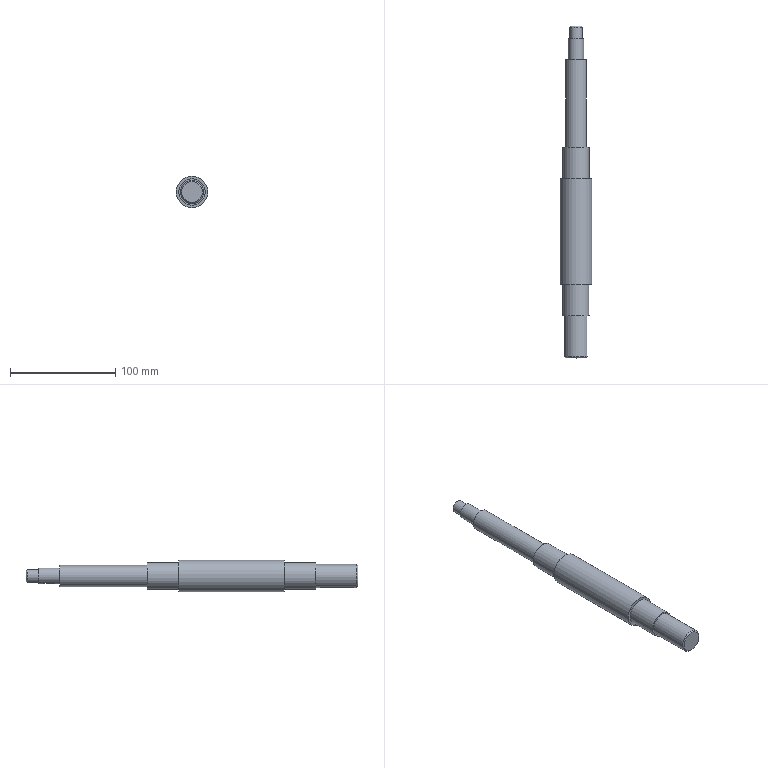Part | NX | features DATUM_CSYS 4, SKETCH 3, DATUM_PLANE 2, EXTRUDE 2, CHAMFER 1, SWP104 1, SYMBOLIC_THREAD 1 | 1 solid | 27 faces | box 30 x 315.25 x 30 mm | volume 145532 mm3 | plane 14 | cylinder 11 | cone 2 | commonest cylinder face diameters 5 x2 6 x2 25 x2 12 x1 15 x1 20 x1
STEP:
#1=CARTESIAN_POINT('',(0.,0.,10.));
#2=VERTEX_POINT('',#1);
#3=CARTESIAN_POINT('',(0.,0.,0.));
#4=DIRECTION('',(0.,1.,0.));
#5=DIRECTION('',(0.,0.,1.));
#6=AXIS2_PLACEMENT_3D('',#3,#4,#5);
#7=CIRCLE('',#6,10.);
#8=EDGE_CURVE('',#2,#2,#7,.F.);
#9=ORIENTED_EDGE('',*,*,#8,.T.);
#10=EDGE_LOOP('',(#9));
#11=FACE_BOUND('',#10,.T.);
#12=CARTESIAN_POINT('',(0.,0.,11.));
#13=DIRECTION('',(0.,1.,0.));
#14=DIRECTION('',(0.,0.,1.));
#15=AXIS2_PLACEMENT_3D('',#12,#13,#14);
#16=PLANE('',#15);
#17=ADVANCED_FACE('',(#11),#16,.F.);
#18=CARTESIAN_POINT('',(0.,315.25,-5.));
#19=VERTEX_POINT('',#18);
#20=CARTESIAN_POINT('',(0.,315.25,0.));
#21=DIRECTION('',(0.,-1.,0.));
#22=DIRECTION('',(0.,0.,-1.));
#23=AXIS2_PLACEMENT_3D('',#20,#21,#22);
#24=CIRCLE('',#23,5.);
#25=EDGE_CURVE('',#19,#19,#24,.F.);
#26=ORIENTED_EDGE('',*,*,#25,.T.);
#27=EDGE_LOOP('',(#26));
#28=FACE_BOUND('',#27,.T.);
#29=CARTESIAN_POINT('',(0.,315.25,0.));
#30=DIRECTION('',(0.,-1.,0.));
#31=DIRECTION('',(0.,0.,-1.));
#32=AXIS2_PLACEMENT_3D('',#29,#30,#31);
#33=PLANE('',#32);
#34=ADVANCED_FACE('',(#28),#33,.F.);
#35=CARTESIAN_POINT('',(0.,314.25,-6.));
#36=VERTEX_POINT('',#35);
#37=CARTESIAN_POINT('',(0.,314.25,0.));
#38=DIRECTION('',(0.,-1.,0.));
#39=DIRECTION('',(0.,0.,-1.));
#40=AXIS2_PLACEMENT_3D('',#37,#38,#39);
#41=CIRCLE('',#40,6.);
#42=EDGE_CURVE('',#36,#36,#41,.T.);
#43=ORIENTED_EDGE('',*,*,#42,.T.);
#44=EDGE_LOOP('',(#43));
#45=FACE_BOUND('',#44,.T.);
#46=CARTESIAN_POINT('',(0.,303.25,-6.));
#47=VERTEX_POINT('',#46);
#48=CARTESIAN_POINT('',(0.,303.25,0.));
#49=DIRECTION('',(0.,-1.,0.));
#50=DIRECTION('',(0.,0.,-1.));
#51=AXIS2_PLACEMENT_3D('',#48,#49,#50);
#52=CIRCLE('',#51,6.);
#53=EDGE_CURVE('',#47,#47,#52,.T.);
#54=ORIENTED_EDGE('',*,*,#53,.F.);
#55=EDGE_LOOP('',(#54));
#56=FACE_BOUND('',#55,.T.);
#57=CARTESIAN_POINT('',(0.,315.25,0.));
#58=DIRECTION('',(0.,-1.,0.));
#59=DIRECTION('',(0.,0.,-1.));
#60=AXIS2_PLACEMENT_3D('',#57,#58,#59);
#61=CYLINDRICAL_SURFACE('',#60,6.);
#62=ADVANCED_FACE('',(#45,#56),#61,.T.);
#63=CARTESIAN_POINT('',(0.,303.25,-7.5));
#64=VERTEX_POINT('',#63);
#65=CARTESIAN_POINT('',(0.,303.25,0.));
#66=DIRECTION('',(0.,-1.,0.));
#67=DIRECTION('',(0.,0.,-1.));
#68=AXIS2_PLACEMENT_3D('',#65,#66,#67);
#69=CIRCLE('',#68,7.5);
#70=EDGE_CURVE('',#64,#64,#69,.T.);
#71=ORIENTED_EDGE('',*,*,#70,.F.);
#72=EDGE_LOOP('',(#71));
#73=FACE_BOUND('',#72,.T.);
#74=ORIENTED_EDGE('',*,*,#53,.T.);
#75=EDGE_LOOP('',(#74));
#76=FACE_BOUND('',#75,.T.);
#77=CARTESIAN_POINT('',(0.,303.25,6.));
#78=DIRECTION('',(0.,-1.,0.));
#79=DIRECTION('',(0.,0.,-1.));
#80=AXIS2_PLACEMENT_3D('',#77,#78,#79);
#81=PLANE('',#80);
#82=ADVANCED_FACE('',(#73,#76),#81,.F.);
#83=CARTESIAN_POINT('',(-2.5,298.25,-7.071));
#84=VERTEX_POINT('',#83);
#85=CARTESIAN_POINT('',(-2.5,289.25,-7.071));
#86=VERTEX_POINT('',#85);
#87=CARTESIAN_POINT('',(-2.5,315.25,-7.071));
#88=DIRECTION('',(0.,-1.,0.));
#89=VECTOR('',#88,1000.);
#90=LINE('',#87,#89);
#91=EDGE_CURVE('',#84,#86,#90,.T.);
#92=ORIENTED_EDGE('',*,*,#91,.T.);
#93=CARTESIAN_POINT('',(2.5,289.25,-7.071));
#94=VERTEX_POINT('',#93);
#95=CARTESIAN_POINT('',(-2.5,289.25,-7.071));
#96=CARTESIAN_POINT('',(-2.5,288.584,-7.071));
#97=CARTESIAN_POINT('',(-1.958,287.298,-7.292));
#98=CARTESIAN_POINT('',(-0.004326,286.476,-7.604));
#99=CARTESIAN_POINT('',(1.96,287.297,-7.292));
#100=CARTESIAN_POINT('',(2.5,288.584,-7.071));
#101=CARTESIAN_POINT('',(2.5,289.25,-7.071));
#102=B_SPLINE_CURVE_WITH_KNOTS('',3,(#95,#96,#97,#98,#99,#100,#101),.UNSPECIFIED.,.F.,.F.,(4,1,1,1,4),(0.,0.001967,0.003935,0.005902,0.00787),.UNSPECIFIED.);
#103=EDGE_CURVE('',#86,#94,#102,.T.);
#104=ORIENTED_EDGE('',*,*,#103,.T.);
#105=CARTESIAN_POINT('',(2.5,298.25,-7.071));
#106=VERTEX_POINT('',#105);
#107=CARTESIAN_POINT('',(2.5,315.25,-7.071));
#108=DIRECTION('',(0.,-1.,0.));
#109=VECTOR('',#108,1000.);
#110=LINE('',#107,#109);
#111=EDGE_CURVE('',#94,#106,#110,.F.);
#112=ORIENTED_EDGE('',*,*,#111,.T.);
#113=CARTESIAN_POINT('',(2.5,298.25,-7.071));
#114=CARTESIAN_POINT('',(2.5,298.916,-7.071));
#115=CARTESIAN_POINT('',(1.958,300.202,-7.292));
#116=CARTESIAN_POINT('',(0.004326,301.024,-7.604));
#117=CARTESIAN_POINT('',(-1.96,300.203,-7.292));
#118=CARTESIAN_POINT('',(-2.5,298.916,-7.071));
#119=CARTESIAN_POINT('',(-2.5,298.25,-7.071));
#120=B_SPLINE_CURVE_WITH_KNOTS('',3,(#113,#114,#115,#116,#117,#118,#119),.UNSPECIFIED.,.F.,.F.,(4,1,1,1,4),(0.,0.001967,0.003935,0.005902,0.00787),.UNSPECIFIED.);
#121=EDGE_CURVE('',#106,#84,#120,.T.);
#122=ORIENTED_EDGE('',*,*,#121,.T.);
#123=EDGE_LOOP('',(#92,#104,#112,#122));
#124=FACE_BOUND('',#123,.T.);
#125=CARTESIAN_POINT('',(0.,283.25,-7.5));
#126=VERTEX_POINT('',#125);
#127=CARTESIAN_POINT('',(0.,283.25,0.));
#128=DIRECTION('',(0.,-1.,0.));
#129=DIRECTION('',(0.,0.,-1.));
#130=AXIS2_PLACEMENT_3D('',#127,#128,#129);
#131=CIRCLE('',#130,7.5);
#132=EDGE_CURVE('',#126,#126,#131,.T.);
#133=ORIENTED_EDGE('',*,*,#132,.F.);
#134=EDGE_LOOP('',(#133));
#135=FACE_BOUND('',#134,.T.);
#136=ORIENTED_EDGE('',*,*,#70,.T.);
#137=EDGE_LOOP('',(#136));
#138=FACE_BOUND('',#137,.T.);
#139=CARTESIAN_POINT('',(0.,315.25,0.));
#140=DIRECTION('',(0.,-1.,0.));
#141=DIRECTION('',(0.,0.,-1.));
#142=AXIS2_PLACEMENT_3D('',#139,#140,#141);
#143=CYLINDRICAL_SURFACE('',#142,7.5);
#144=ADVANCED_FACE('',(#124,#135,#138),#143,.T.);
#145=CARTESIAN_POINT('',(0.,283.25,-10.));
#146=VERTEX_POINT('',#145);
#147=CARTESIAN_POINT('',(0.,283.25,0.));
#148=DIRECTION('',(0.,-1.,0.));
#149=DIRECTION('',(0.,0.,-1.));
#150=AXIS2_PLACEMENT_3D('',#147,#148,#149);
#151=CIRCLE('',#150,10.);
#152=EDGE_CURVE('',#146,#146,#151,.T.);
#153=ORIENTED_EDGE('',*,*,#152,.F.);
#154=EDGE_LOOP('',(#153));
#155=FACE_BOUND('',#154,.T.);
#156=ORIENTED_EDGE('',*,*,#132,.T.);
#157=EDGE_LOOP('',(#156));
#158=FACE_BOUND('',#157,.T.);
#159=CARTESIAN_POINT('',(0.,283.25,7.5));
#160=DIRECTION('',(0.,-1.,0.));
#161=DIRECTION('',(0.,0.,-1.));
#162=AXIS2_PLACEMENT_3D('',#159,#160,#161);
#163=PLANE('',#162);
#164=ADVANCED_FACE('',(#155,#158),#163,.F.);
#165=CARTESIAN_POINT('',(0.,200.,-10.));
#166=VERTEX_POINT('',#165);
#167=CARTESIAN_POINT('',(0.,200.,0.));
#168=DIRECTION('',(0.,-1.,0.));
#169=DIRECTION('',(0.,0.,-1.));
#170=AXIS2_PLACEMENT_3D('',#167,#168,#169);
#171=CIRCLE('',#170,10.);
#172=EDGE_CURVE('',#166,#166,#171,.T.);
#173=ORIENTED_EDGE('',*,*,#172,.F.);
#174=EDGE_LOOP('',(#173));
#175=FACE_BOUND('',#174,.T.);
#176=ORIENTED_EDGE('',*,*,#152,.T.);
#177=EDGE_LOOP('',(#176));
#178=FACE_BOUND('',#177,.T.);
#179=CARTESIAN_POINT('',(0.,315.25,0.));
#180=DIRECTION('',(0.,-1.,0.));
#181=DIRECTION('',(0.,0.,-1.));
#182=AXIS2_PLACEMENT_3D('',#179,#180,#181);
#183=CYLINDRICAL_SURFACE('',#182,10.);
#184=ADVANCED_FACE('',(#175,#178),#183,.T.);
#185=CARTESIAN_POINT('',(0.,200.,-12.5));
#186=VERTEX_POINT('',#185);
#187=CARTESIAN_POINT('',(0.,200.,0.));
#188=DIRECTION('',(0.,-1.,0.));
#189=DIRECTION('',(0.,0.,-1.));
#190=AXIS2_PLACEMENT_3D('',#187,#188,#189);
#191=CIRCLE('',#190,12.5);
#192=EDGE_CURVE('',#186,#186,#191,.T.);
#193=ORIENTED_EDGE('',*,*,#192,.F.);
#194=EDGE_LOOP('',(#193));
#195=FACE_BOUND('',#194,.T.);
#196=ORIENTED_EDGE('',*,*,#172,.T.);
#197=EDGE_LOOP('',(#196));
#198=FACE_BOUND('',#197,.T.);
#199=CARTESIAN_POINT('',(0.,200.,10.));
#200=DIRECTION('',(0.,-1.,0.));
#201=DIRECTION('',(0.,0.,-1.));
#202=AXIS2_PLACEMENT_3D('',#199,#200,#201);
#203=PLANE('',#202);
#204=ADVANCED_FACE('',(#195,#198),#203,.F.);
#205=CARTESIAN_POINT('',(0.,170.,-12.5));
#206=VERTEX_POINT('',#205);
#207=CARTESIAN_POINT('',(0.,170.,0.));
#208=DIRECTION('',(0.,-1.,0.));
#209=DIRECTION('',(0.,0.,-1.));
#210=AXIS2_PLACEMENT_3D('',#207,#208,#209);
#211=CIRCLE('',#210,12.5);
#212=EDGE_CURVE('',#206,#206,#211,.T.);
#213=ORIENTED_EDGE('',*,*,#212,.F.);
#214=EDGE_LOOP('',(#213));
#215=FACE_BOUND('',#214,.T.);
#216=ORIENTED_EDGE('',*,*,#192,.T.);
#217=EDGE_LOOP('',(#216));
#218=FACE_BOUND('',#217,.T.);
#219=CARTESIAN_POINT('',(0.,315.25,0.));
#220=DIRECTION('',(0.,-1.,0.));
#221=DIRECTION('',(0.,0.,-1.));
#222=AXIS2_PLACEMENT_3D('',#219,#220,#221);
#223=CYLINDRICAL_SURFACE('',#222,12.5);
#224=ADVANCED_FACE('',(#215,#218),#223,.T.);
#225=CARTESIAN_POINT('',(0.,170.,-15.));
#226=VERTEX_POINT('',#225);
#227=CARTESIAN_POINT('',(0.,170.,0.));
#228=DIRECTION('',(0.,-1.,0.));
#229=DIRECTION('',(0.,0.,-1.));
#230=AXIS2_PLACEMENT_3D('',#227,#228,#229);
#231=CIRCLE('',#230,15.);
#232=EDGE_CURVE('',#226,#226,#231,.T.);
#233=ORIENTED_EDGE('',*,*,#232,.F.);
#234=EDGE_LOOP('',(#233));
#235=FACE_BOUND('',#234,.T.);
#236=ORIENTED_EDGE('',*,*,#212,.T.);
#237=EDGE_LOOP('',(#236));
#238=FACE_BOUND('',#237,.T.);
#239=CARTESIAN_POINT('',(0.,170.,12.5));
#240=DIRECTION('',(0.,-1.,0.));
#241=DIRECTION('',(0.,0.,-1.));
#242=AXIS2_PLACEMENT_3D('',#239,#240,#241);
#243=PLANE('',#242);
#244=ADVANCED_FACE('',(#235,#238),#243,.F.);
#245=CARTESIAN_POINT('',(0.,70.,-15.));
#246=VERTEX_POINT('',#245);
#247=CARTESIAN_POINT('',(0.,70.,0.));
#248=DIRECTION('',(0.,-1.,0.));
#249=DIRECTION('',(0.,0.,-1.));
#250=AXIS2_PLACEMENT_3D('',#247,#248,#249);
#251=CIRCLE('',#250,15.);
#252=EDGE_CURVE('',#246,#246,#251,.T.);
#253=ORIENTED_EDGE('',*,*,#252,.F.);
#254=EDGE_LOOP('',(#253));
#255=FACE_BOUND('',#254,.T.);
#256=ORIENTED_EDGE('',*,*,#232,.T.);
#257=EDGE_LOOP('',(#256));
#258=FACE_BOUND('',#257,.T.);
#259=CARTESIAN_POINT('',(0.,315.25,0.));
#260=DIRECTION('',(0.,-1.,0.));
#261=DIRECTION('',(0.,0.,-1.));
#262=AXIS2_PLACEMENT_3D('',#259,#260,#261);
#263=CYLINDRICAL_SURFACE('',#262,15.);
#264=ADVANCED_FACE('',(#255,#258),#263,.T.);
#265=CARTESIAN_POINT('',(0.,70.,-12.5));
#266=VERTEX_POINT('',#265);
#267=CARTESIAN_POINT('',(0.,70.,0.));
#268=DIRECTION('',(0.,-1.,0.));
#269=DIRECTION('',(0.,0.,-1.));
#270=AXIS2_PLACEMENT_3D('',#267,#268,#269);
#271=CIRCLE('',#270,12.5);
#272=EDGE_CURVE('',#266,#266,#271,.T.);
#273=ORIENTED_EDGE('',*,*,#272,.F.);
#274=EDGE_LOOP('',(#273));
#275=FACE_BOUND('',#274,.T.);
#276=ORIENTED_EDGE('',*,*,#252,.T.);
#277=EDGE_LOOP('',(#276));
#278=FACE_BOUND('',#277,.T.);
#279=CARTESIAN_POINT('',(0.,70.,15.));
#280=DIRECTION('',(0.,1.,0.));
#281=DIRECTION('',(0.,0.,1.));
#282=AXIS2_PLACEMENT_3D('',#279,#280,#281);
#283=PLANE('',#282);
#284=ADVANCED_FACE('',(#275,#278),#283,.F.);
#285=CARTESIAN_POINT('',(0.,40.,-12.5));
#286=VERTEX_POINT('',#285);
#287=CARTESIAN_POINT('',(0.,40.,0.));
#288=DIRECTION('',(0.,-1.,0.));
#289=DIRECTION('',(0.,0.,-1.));
#290=AXIS2_PLACEMENT_3D('',#287,#288,#289);
#291=CIRCLE('',#290,12.5);
#292=EDGE_CURVE('',#286,#286,#291,.T.);
#293=ORIENTED_EDGE('',*,*,#292,.F.);
#294=EDGE_LOOP('',(#293));
#295=FACE_BOUND('',#294,.T.);
#296=ORIENTED_EDGE('',*,*,#272,.T.);
#297=EDGE_LOOP('',(#296));
#298=FACE_BOUND('',#297,.T.);
#299=CARTESIAN_POINT('',(0.,315.25,0.));
#300=DIRECTION('',(0.,-1.,0.));
#301=DIRECTION('',(0.,0.,-1.));
#302=AXIS2_PLACEMENT_3D('',#299,#300,#301);
#303=CYLINDRICAL_SURFACE('',#302,12.5);
#304=ADVANCED_FACE('',(#295,#298),#303,.T.);
#305=CARTESIAN_POINT('',(0.,40.,-11.));
#306=VERTEX_POINT('',#305);
#307=CARTESIAN_POINT('',(0.,40.,0.));
#308=DIRECTION('',(0.,-1.,0.));
#309=DIRECTION('',(0.,0.,-1.));
#310=AXIS2_PLACEMENT_3D('',#307,#308,#309);
#311=CIRCLE('',#310,11.);
#312=EDGE_CURVE('',#306,#306,#311,.T.);
#313=ORIENTED_EDGE('',*,*,#312,.F.);
#314=EDGE_LOOP('',(#313));
#315=FACE_BOUND('',#314,.T.);
#316=ORIENTED_EDGE('',*,*,#292,.T.);
#317=EDGE_LOOP('',(#316));
#318=FACE_BOUND('',#317,.T.);
#319=CARTESIAN_POINT('',(0.,40.,12.5));
#320=DIRECTION('',(0.,1.,0.));
#321=DIRECTION('',(0.,0.,1.));
#322=AXIS2_PLACEMENT_3D('',#319,#320,#321);
#323=PLANE('',#322);
#324=ADVANCED_FACE('',(#315,#318),#323,.F.);
#325=CARTESIAN_POINT('',(0.,1.,11.));
#326=VERTEX_POINT('',#325);
#327=CARTESIAN_POINT('',(0.,1.,0.));
#328=DIRECTION('',(0.,1.,0.));
#329=DIRECTION('',(0.,0.,1.));
#330=AXIS2_PLACEMENT_3D('',#327,#328,#329);
#331=CIRCLE('',#330,11.);
#332=EDGE_CURVE('',#326,#326,#331,.T.);
#333=ORIENTED_EDGE('',*,*,#332,.T.);
#334=EDGE_LOOP('',(#333));
#335=FACE_BOUND('',#334,.T.);
#336=CARTESIAN_POINT('',(-3.,33.,-10.583));
#337=VERTEX_POINT('',#336);
#338=CARTESIAN_POINT('',(-3.,7.,-10.583));
#339=VERTEX_POINT('',#338);
#340=CARTESIAN_POINT('',(-3.,315.25,-10.583));
#341=DIRECTION('',(0.,-1.,0.));
#342=VECTOR('',#341,1000.);
#343=LINE('',#340,#342);
#344=EDGE_CURVE('',#337,#339,#343,.T.);
#345=ORIENTED_EDGE('',*,*,#344,.T.);
#346=CARTESIAN_POINT('',(3.,7.,-10.583));
#347=VERTEX_POINT('',#346);
#348=CARTESIAN_POINT('',(-3.,7.,-10.583));
#349=CARTESIAN_POINT('',(-3.,6.203,-10.583));
#350=CARTESIAN_POINT('',(-2.35,4.656,-10.796));
#351=CARTESIAN_POINT('',(-0.004455,3.673,-11.102));
#352=CARTESIAN_POINT('',(2.351,4.654,-10.796));
#353=CARTESIAN_POINT('',(3.,6.203,-10.583));
#354=CARTESIAN_POINT('',(3.,7.,-10.583));
#355=B_SPLINE_CURVE_WITH_KNOTS('',3,(#348,#349,#350,#351,#352,#353,#354),.UNSPECIFIED.,.F.,.F.,(4,1,1,1,4),(0.,0.002355,0.004711,0.007066,0.009421),.UNSPECIFIED.);
#356=EDGE_CURVE('',#339,#347,#355,.T.);
#357=ORIENTED_EDGE('',*,*,#356,.T.);
#358=CARTESIAN_POINT('',(3.,33.,-10.583));
#359=VERTEX_POINT('',#358);
#360=CARTESIAN_POINT('',(3.,315.25,-10.583));
#361=DIRECTION('',(0.,-1.,0.));
#362=VECTOR('',#361,1000.);
#363=LINE('',#360,#362);
#364=EDGE_CURVE('',#347,#359,#363,.F.);
#365=ORIENTED_EDGE('',*,*,#364,.T.);
#366=CARTESIAN_POINT('',(3.,33.,-10.583));
#367=CARTESIAN_POINT('',(3.,33.797,-10.583));
#368=CARTESIAN_POINT('',(2.35,35.344,-10.796));
#369=CARTESIAN_POINT('',(0.004455,36.327,-11.102));
#370=CARTESIAN_POINT('',(-2.351,35.346,-10.796));
#371=CARTESIAN_POINT('',(-3.,33.797,-10.583));
#372=CARTESIAN_POINT('',(-3.,33.,-10.583));
#373=B_SPLINE_CURVE_WITH_KNOTS('',3,(#366,#367,#368,#369,#370,#371,#372),.UNSPECIFIED.,.F.,.F.,(4,1,1,1,4),(0.,0.002355,0.004711,0.007066,0.009421),.UNSPECIFIED.);
#374=EDGE_CURVE('',#359,#337,#373,.T.);
#375=ORIENTED_EDGE('',*,*,#374,.T.);
#376=EDGE_LOOP('',(#345,#357,#365,#375));
#377=FACE_BOUND('',#376,.T.);
#378=ORIENTED_EDGE('',*,*,#312,.T.);
#379=EDGE_LOOP('',(#378));
#380=FACE_BOUND('',#379,.T.);
#381=CARTESIAN_POINT('',(0.,315.25,0.));
#382=DIRECTION('',(0.,-1.,0.));
#383=DIRECTION('',(0.,0.,-1.));
#384=AXIS2_PLACEMENT_3D('',#381,#382,#383);
#385=CYLINDRICAL_SURFACE('',#384,11.);
#386=ADVANCED_FACE('',(#335,#377,#380),#385,.T.);
#387=CARTESIAN_POINT('',(-2.5,298.25,-4.5));
#388=VERTEX_POINT('',#387);
#389=CARTESIAN_POINT('',(-2.5,298.25,-4.5));
#390=DIRECTION('',(0.,0.,-1.));
#391=VECTOR('',#390,1000.);
#392=LINE('',#389,#391);
#393=EDGE_CURVE('',#84,#388,#392,.F.);
#394=ORIENTED_EDGE('',*,*,#393,.T.);
#395=CARTESIAN_POINT('',(-2.5,289.25,-4.5));
#396=VERTEX_POINT('',#395);
#397=CARTESIAN_POINT('',(-2.5,289.25,-4.5));
#398=DIRECTION('',(0.,1.,0.));
#399=VECTOR('',#398,1000.);
#400=LINE('',#397,#399);
#401=EDGE_CURVE('',#388,#396,#400,.F.);
#402=ORIENTED_EDGE('',*,*,#401,.T.);
#403=CARTESIAN_POINT('',(-2.5,289.25,-4.5));
#404=DIRECTION('',(0.,0.,-1.));
#405=VECTOR('',#404,1000.);
#406=LINE('',#403,#405);
#407=EDGE_CURVE('',#86,#396,#406,.F.);
#408=ORIENTED_EDGE('',*,*,#407,.F.);
#409=ORIENTED_EDGE('',*,*,#91,.F.);
#410=EDGE_LOOP('',(#394,#402,#408,#409));
#411=FACE_BOUND('',#410,.T.);
#412=CARTESIAN_POINT('',(-2.5,289.25,-4.5));
#413=DIRECTION('',(-1.,0.,0.));
#414=DIRECTION('',(0.,-1.,0.));
#415=AXIS2_PLACEMENT_3D('',#412,#413,#414);
#416=PLANE('',#415);
#417=ADVANCED_FACE('',(#411),#416,.F.);
#418=CARTESIAN_POINT('',(2.5,298.25,-4.5));
#419=VERTEX_POINT('',#418);
#420=CARTESIAN_POINT('',(2.5,298.25,-4.5));
#421=DIRECTION('',(0.,0.,-1.));
#422=VECTOR('',#421,1000.);
#423=LINE('',#420,#422);
#424=EDGE_CURVE('',#106,#419,#423,.F.);
#425=ORIENTED_EDGE('',*,*,#424,.T.);
#426=CARTESIAN_POINT('',(0.,298.25,-4.5));
#427=DIRECTION('',(0.,0.,-1.));
#428=DIRECTION('',(1.,0.,0.));
#429=AXIS2_PLACEMENT_3D('',#426,#427,#428);
#430=CIRCLE('',#429,2.5);
#431=EDGE_CURVE('',#419,#388,#430,.F.);
#432=ORIENTED_EDGE('',*,*,#431,.T.);
#433=ORIENTED_EDGE('',*,*,#393,.F.);
#434=ORIENTED_EDGE('',*,*,#121,.F.);
#435=EDGE_LOOP('',(#425,#432,#433,#434));
#436=FACE_BOUND('',#435,.T.);
#437=CARTESIAN_POINT('',(0.,298.25,-4.5));
#438=DIRECTION('',(0.,0.,-1.));
#439=DIRECTION('',(-1.,0.,0.));
#440=AXIS2_PLACEMENT_3D('',#437,#438,#439);
#441=CYLINDRICAL_SURFACE('',#440,2.5);
#442=ADVANCED_FACE('',(#436),#441,.F.);
#443=CARTESIAN_POINT('',(2.5,289.25,-4.5));
#444=VERTEX_POINT('',#443);
#445=CARTESIAN_POINT('',(2.5,289.25,-4.5));
#446=DIRECTION('',(0.,0.,-1.));
#447=VECTOR('',#446,1000.);
#448=LINE('',#445,#447);
#449=EDGE_CURVE('',#94,#444,#448,.F.);
#450=ORIENTED_EDGE('',*,*,#449,.T.);
#451=CARTESIAN_POINT('',(2.5,298.25,-4.5));
#452=DIRECTION('',(0.,-1.,0.));
#453=VECTOR('',#452,1000.);
#454=LINE('',#451,#453);
#455=EDGE_CURVE('',#444,#419,#454,.F.);
#456=ORIENTED_EDGE('',*,*,#455,.T.);
#457=ORIENTED_EDGE('',*,*,#424,.F.);
#458=ORIENTED_EDGE('',*,*,#111,.F.);
#459=EDGE_LOOP('',(#450,#456,#457,#458));
#460=FACE_BOUND('',#459,.T.);
#461=CARTESIAN_POINT('',(2.5,298.25,-4.5));
#462=DIRECTION('',(1.,0.,0.));
#463=DIRECTION('',(0.,1.,0.));
#464=AXIS2_PLACEMENT_3D('',#461,#462,#463);
#465=PLANE('',#464);
#466=ADVANCED_FACE('',(#460),#465,.F.);
#467=ORIENTED_EDGE('',*,*,#407,.T.);
#468=CARTESIAN_POINT('',(0.,289.25,-4.5));
#469=DIRECTION('',(0.,0.,-1.));
#470=DIRECTION('',(1.,0.,0.));
#471=AXIS2_PLACEMENT_3D('',#468,#469,#470);
#472=CIRCLE('',#471,2.5);
#473=EDGE_CURVE('',#396,#444,#472,.F.);
#474=ORIENTED_EDGE('',*,*,#473,.T.);
#475=ORIENTED_EDGE('',*,*,#449,.F.);
#476=ORIENTED_EDGE('',*,*,#103,.F.);
#477=EDGE_LOOP('',(#467,#474,#475,#476));
#478=FACE_BOUND('',#477,.T.);
#479=CARTESIAN_POINT('',(0.,289.25,-4.5));
#480=DIRECTION('',(0.,0.,-1.));
#481=DIRECTION('',(-1.,0.,0.));
#482=AXIS2_PLACEMENT_3D('',#479,#480,#481);
#483=CYLINDRICAL_SURFACE('',#482,2.5);
#484=ADVANCED_FACE('',(#478),#483,.F.);
#485=ORIENTED_EDGE('',*,*,#401,.F.);
#486=ORIENTED_EDGE('',*,*,#431,.F.);
#487=ORIENTED_EDGE('',*,*,#455,.F.);
#488=ORIENTED_EDGE('',*,*,#473,.F.);
#489=EDGE_LOOP('',(#485,#486,#487,#488));
#490=FACE_BOUND('',#489,.T.);
#491=CARTESIAN_POINT('',(0.,298.25,-4.5));
#492=DIRECTION('',(0.,0.,-1.));
#493=DIRECTION('',(-1.,0.,0.));
#494=AXIS2_PLACEMENT_3D('',#491,#492,#493);
#495=PLANE('',#494);
#496=ADVANCED_FACE('',(#490),#495,.T.);
#497=CARTESIAN_POINT('',(-3.,33.,-7.5));
#498=VERTEX_POINT('',#497);
#499=CARTESIAN_POINT('',(-3.,33.,-7.5));
#500=DIRECTION('',(0.,0.,-1.));
#501=VECTOR('',#500,1000.);
#502=LINE('',#499,#501);
#503=EDGE_CURVE('',#337,#498,#502,.F.);
#504=ORIENTED_EDGE('',*,*,#503,.T.);
#505=CARTESIAN_POINT('',(-3.,7.,-7.5));
#506=VERTEX_POINT('',#505);
#507=CARTESIAN_POINT('',(-3.,7.,-7.5));
#508=DIRECTION('',(0.,1.,0.));
#509=VECTOR('',#508,1000.);
#510=LINE('',#507,#509);
#511=EDGE_CURVE('',#498,#506,#510,.F.);
#512=ORIENTED_EDGE('',*,*,#511,.T.);
#513=CARTESIAN_POINT('',(-3.,7.,-7.5));
#514=DIRECTION('',(0.,0.,-1.));
#515=VECTOR('',#514,1000.);
#516=LINE('',#513,#515);
#517=EDGE_CURVE('',#339,#506,#516,.F.);
#518=ORIENTED_EDGE('',*,*,#517,.F.);
#519=ORIENTED_EDGE('',*,*,#344,.F.);
#520=EDGE_LOOP('',(#504,#512,#518,#519));
#521=FACE_BOUND('',#520,.T.);
#522=CARTESIAN_POINT('',(-3.,7.,-7.5));
#523=DIRECTION('',(-1.,0.,0.));
#524=DIRECTION('',(0.,-1.,0.));
#525=AXIS2_PLACEMENT_3D('',#522,#523,#524);
#526=PLANE('',#525);
#527=ADVANCED_FACE('',(#521),#526,.F.);
#528=CARTESIAN_POINT('',(3.,33.,-7.5));
#529=VERTEX_POINT('',#528);
#530=CARTESIAN_POINT('',(3.,33.,-7.5));
#531=DIRECTION('',(0.,0.,-1.));
#532=VECTOR('',#531,1000.);
#533=LINE('',#530,#532);
#534=EDGE_CURVE('',#359,#529,#533,.F.);
#535=ORIENTED_EDGE('',*,*,#534,.T.);
#536=CARTESIAN_POINT('',(0.,33.,-7.5));
#537=DIRECTION('',(0.,0.,-1.));
#538=DIRECTION('',(1.,0.,0.));
#539=AXIS2_PLACEMENT_3D('',#536,#537,#538);
#540=CIRCLE('',#539,3.);
#541=EDGE_CURVE('',#529,#498,#540,.F.);
#542=ORIENTED_EDGE('',*,*,#541,.T.);
#543=ORIENTED_EDGE('',*,*,#503,.F.);
#544=ORIENTED_EDGE('',*,*,#374,.F.);
#545=EDGE_LOOP('',(#535,#542,#543,#544));
#546=FACE_BOUND('',#545,.T.);
#547=CARTESIAN_POINT('',(0.,33.,-7.5));
#548=DIRECTION('',(0.,0.,-1.));
#549=DIRECTION('',(-1.,0.,0.));
#550=AXIS2_PLACEMENT_3D('',#547,#548,#549);
#551=CYLINDRICAL_SURFACE('',#550,3.);
#552=ADVANCED_FACE('',(#546),#551,.F.);
#553=CARTESIAN_POINT('',(3.,7.,-7.5));
#554=VERTEX_POINT('',#553);
#555=CARTESIAN_POINT('',(3.,7.,-7.5));
#556=DIRECTION('',(0.,0.,-1.));
#557=VECTOR('',#556,1000.);
#558=LINE('',#555,#557);
#559=EDGE_CURVE('',#347,#554,#558,.F.);
#560=ORIENTED_EDGE('',*,*,#559,.T.);
#561=CARTESIAN_POINT('',(3.,33.,-7.5));
#562=DIRECTION('',(0.,-1.,0.));
#563=VECTOR('',#562,1000.);
#564=LINE('',#561,#563);
#565=EDGE_CURVE('',#554,#529,#564,.F.);
#566=ORIENTED_EDGE('',*,*,#565,.T.);
#567=ORIENTED_EDGE('',*,*,#534,.F.);
#568=ORIENTED_EDGE('',*,*,#364,.F.);
#569=EDGE_LOOP('',(#560,#566,#567,#568));
#570=FACE_BOUND('',#569,.T.);
#571=CARTESIAN_POINT('',(3.,33.,-7.5));
#572=DIRECTION('',(1.,0.,0.));
#573=DIRECTION('',(0.,1.,0.));
#574=AXIS2_PLACEMENT_3D('',#571,#572,#573);
#575=PLANE('',#574);
#576=ADVANCED_FACE('',(#570),#575,.F.);
#577=ORIENTED_EDGE('',*,*,#517,.T.);
#578=CARTESIAN_POINT('',(0.,7.,-7.5));
#579=DIRECTION('',(0.,0.,-1.));
#580=DIRECTION('',(1.,0.,0.));
#581=AXIS2_PLACEMENT_3D('',#578,#579,#580);
#582=CIRCLE('',#581,3.);
#583=EDGE_CURVE('',#506,#554,#582,.F.);
#584=ORIENTED_EDGE('',*,*,#583,.T.);
#585=ORIENTED_EDGE('',*,*,#559,.F.);
#586=ORIENTED_EDGE('',*,*,#356,.F.);
#587=EDGE_LOOP('',(#577,#584,#585,#586));
#588=FACE_BOUND('',#587,.T.);
#589=CARTESIAN_POINT('',(0.,7.,-7.5));
#590=DIRECTION('',(0.,0.,-1.));
#591=DIRECTION('',(-1.,0.,0.));
#592=AXIS2_PLACEMENT_3D('',#589,#590,#591);
#593=CYLINDRICAL_SURFACE('',#592,3.);
#594=ADVANCED_FACE('',(#588),#593,.F.);
#595=ORIENTED_EDGE('',*,*,#511,.F.);
#596=ORIENTED_EDGE('',*,*,#541,.F.);
#597=ORIENTED_EDGE('',*,*,#565,.F.);
#598=ORIENTED_EDGE('',*,*,#583,.F.);
#599=EDGE_LOOP('',(#595,#596,#597,#598));
#600=FACE_BOUND('',#599,.T.);
#601=CARTESIAN_POINT('',(0.,33.,-7.5));
#602=DIRECTION('',(0.,0.,-1.));
#603=DIRECTION('',(-1.,0.,0.));
#604=AXIS2_PLACEMENT_3D('',#601,#602,#603);
#605=PLANE('',#604);
#606=ADVANCED_FACE('',(#600),#605,.T.);
#607=ORIENTED_EDGE('',*,*,#25,.F.);
#608=EDGE_LOOP('',(#607));
#609=FACE_BOUND('',#608,.T.);
#610=ORIENTED_EDGE('',*,*,#42,.F.);
#611=EDGE_LOOP('',(#610));
#612=FACE_BOUND('',#611,.T.);
#613=CARTESIAN_POINT('',(0.,314.25,0.));
#614=DIRECTION('',(0.,-1.,0.));
#615=DIRECTION('',(0.,0.,-1.));
#616=AXIS2_PLACEMENT_3D('',#613,#614,#615);
#617=CONICAL_SURFACE('',#616,6.,0.7854);
#618=ADVANCED_FACE('',(#609,#612),#617,.T.);
#619=ORIENTED_EDGE('',*,*,#332,.F.);
#620=EDGE_LOOP('',(#619));
#621=FACE_BOUND('',#620,.T.);
#622=ORIENTED_EDGE('',*,*,#8,.F.);
#623=EDGE_LOOP('',(#622));
#624=FACE_BOUND('',#623,.T.);
#625=CARTESIAN_POINT('',(0.,0.,0.));
#626=DIRECTION('',(0.,1.,0.));
#627=DIRECTION('',(0.,0.,1.));
#628=AXIS2_PLACEMENT_3D('',#625,#626,#627);
#629=CONICAL_SURFACE('',#628,10.,0.7854);
#630=ADVANCED_FACE('',(#621,#624),#629,.T.);
#631=CLOSED_SHELL('',(#17,#34,#62,#82,#144,#164,#184,#204,#224,#244,#264,#284,#304,#324,#386,#417,#442,#466,#484,#496,#527,#552,#576,#594,#606,#618,#630));
#632=MANIFOLD_SOLID_BREP('',#631);
#633=(LENGTH_UNIT()NAMED_UNIT(*)SI_UNIT(.MILLI.,.METRE.));
#634=UNCERTAINTY_MEASURE_WITH_UNIT(LENGTH_MEASURE(0.0508),#633,'','');
#635=(NAMED_UNIT(*)PLANE_ANGLE_UNIT()SI_UNIT($,.RADIAN.));
#636=(NAMED_UNIT(*)SI_UNIT($,.STERADIAN.)SOLID_ANGLE_UNIT());
#637=(GEOMETRIC_REPRESENTATION_CONTEXT(3)GLOBAL_UNCERTAINTY_ASSIGNED_CONTEXT((#634))GLOBAL_UNIT_ASSIGNED_CONTEXT((#633,#635,#636))REPRESENTATION_CONTEXT('',''));
#638=ADVANCED_BREP_SHAPE_REPRESENTATION('',(#632),#637);